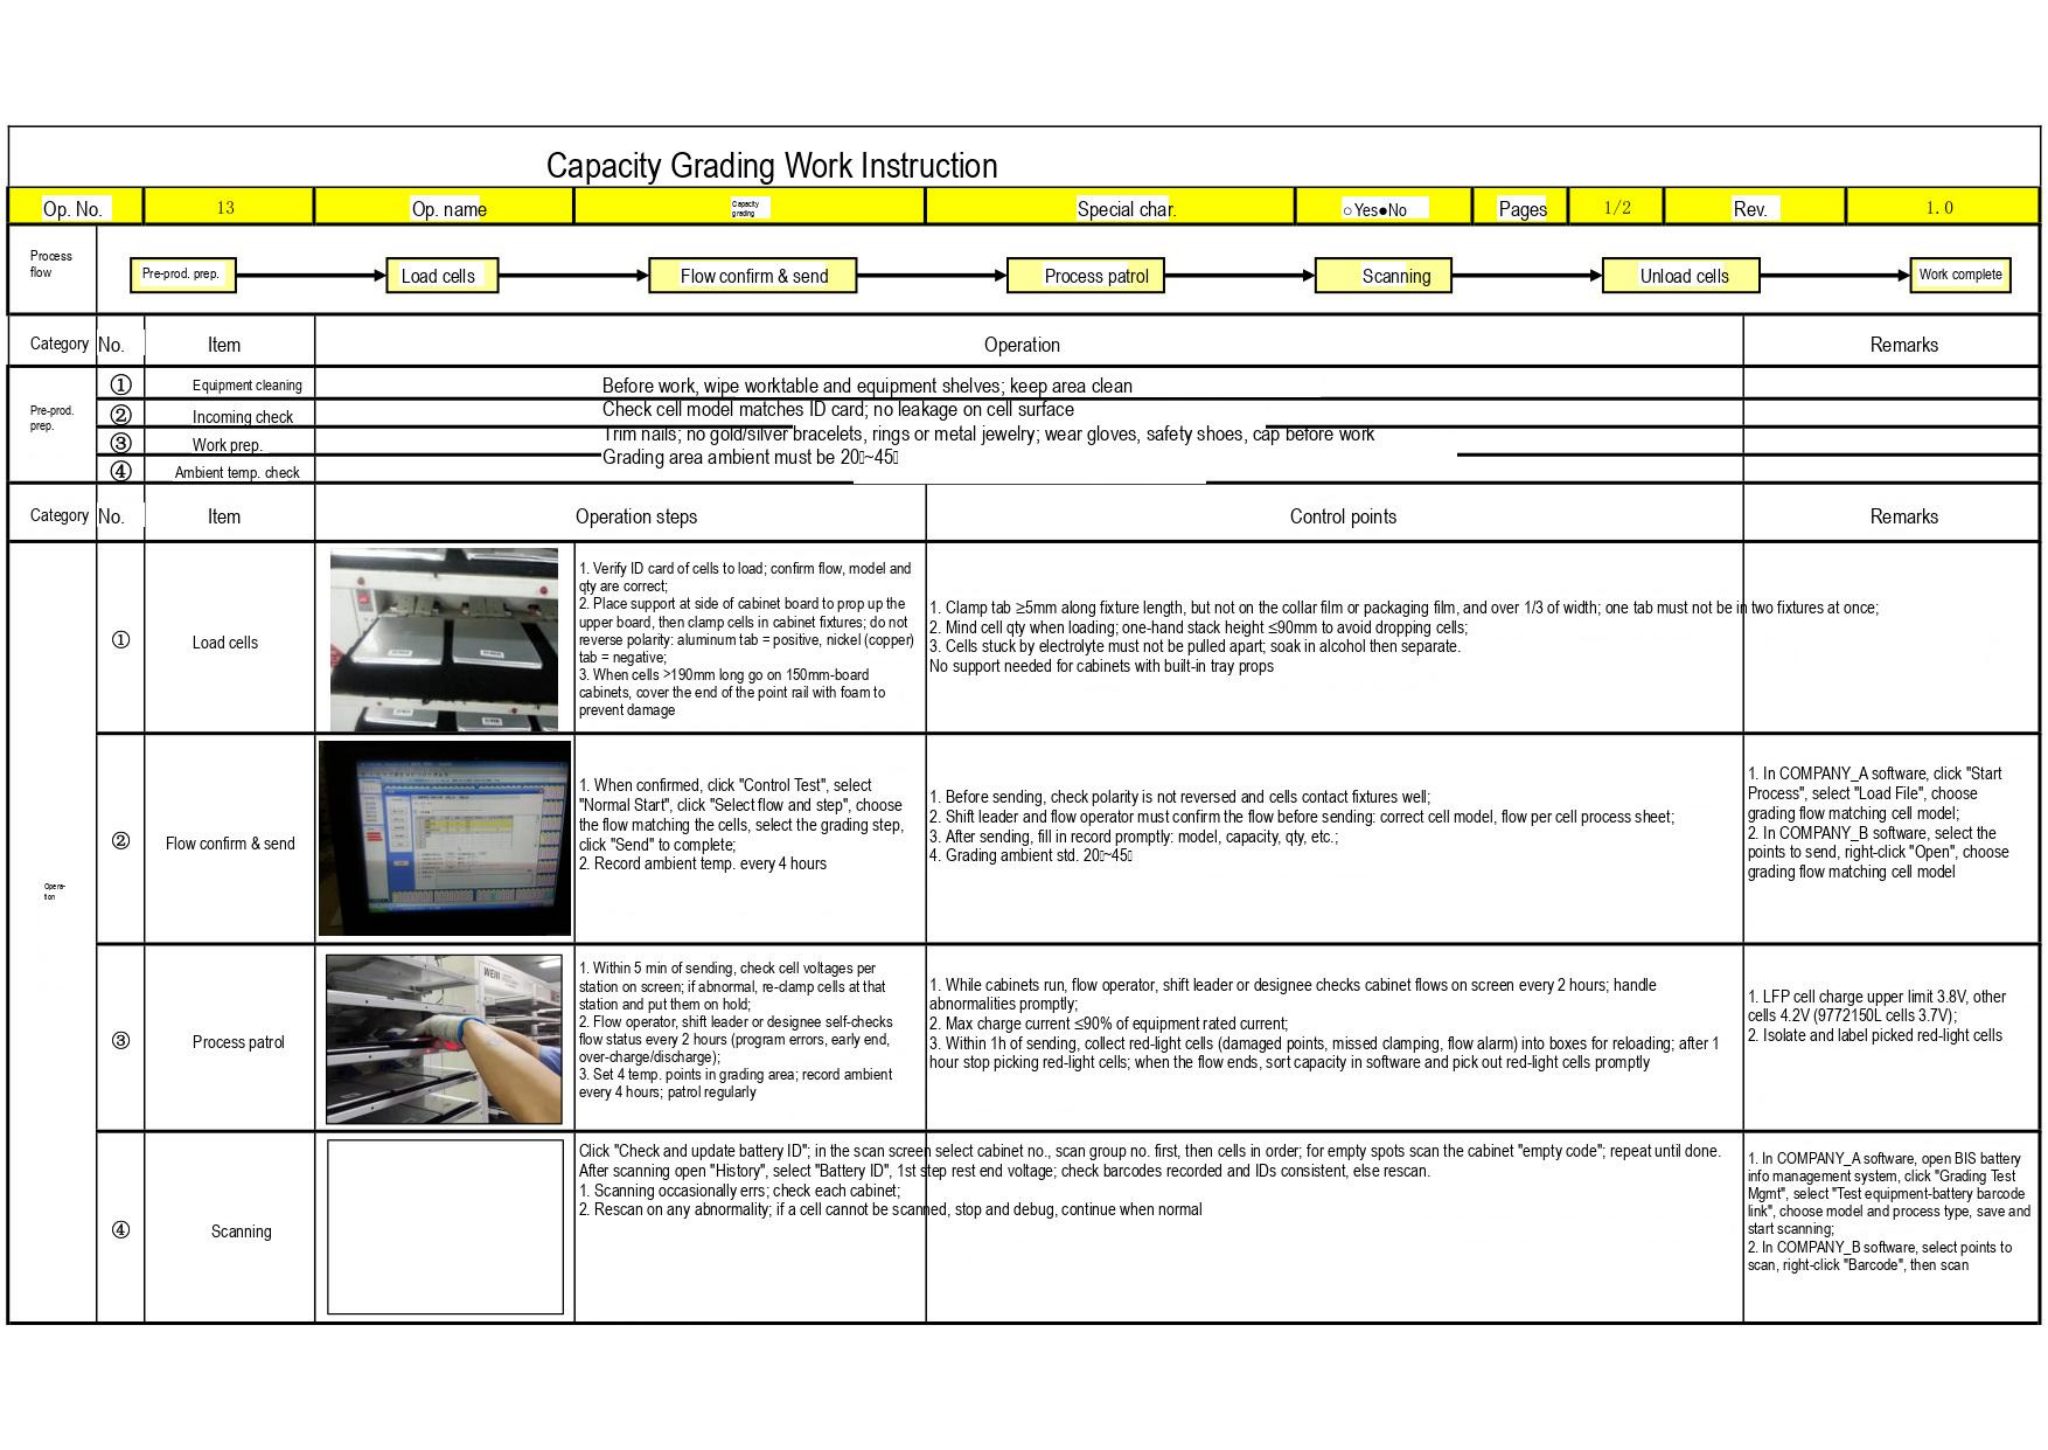# Capacity Grading Work Instruction

| Op. No. | 13 | Op. name | Capacity grading | Special char. | ○Yes●No | Pages | 1/2 | Rev. | 1.0 |
|---|---|---|---|---|---|---|---|---|---|

Process flow: Pre-prod. prep. → Load cells → Flow confirm & send → Process patrol → Scanning → Unload cells → Work complete

| Category | No. | Item | Operation | Remarks |
|---|---|---|---|---|
| Pre-prod. prep. | ① | Equipment cleaning | Before work, wipe worktable and equipment shelves; keep area clean | |
| | ② | Incoming check | Check cell model matches ID card; no leakage on cell surface | |
| | ③ | Work prep. | Trim nails; no gold/silver bracelets, rings or metal jewelry; wear gloves, safety shoes, cap before work | |
| | ④ | Ambient temp. check | Grading area ambient must be 20~45 | |

| Category | No. | Item | Operation steps | | Control points | Remarks |
|---|---|---|---|---|---|---|
| Operation | ① | Load cells | | 1. Verify ID card of cells to load; confirm flow, model and qty are correct;<br>2. Place support at side of cabinet board to prop up the upper board, then clamp cells in cabinet fixtures; do not reverse polarity: aluminum tab = positive, nickel (copper) tab = negative;<br>3. When cells >190mm long go on 150mm-board cabinets, cover the end of the point rail with foam to prevent damage | 1. Clamp tab ≥5mm along fixture length, but not on the collar film or packaging film, and over 1/3 of width; one tab must not be in two fixtures at once;<br>2. Mind cell qty when loading; one-hand stack height ≤90mm to avoid dropping cells;<br>3. Cells stuck by electrolyte must not be pulled apart; soak in alcohol then separate.<br>No support needed for cabinets with built-in tray props | |
| | ② | Flow confirm & send | | 1. When confirmed, click "Control Test", select "Normal Start", click "Select flow and step", choose the flow matching the cells, select the grading step, click "Send" to complete;<br>2. Record ambient temp. every 4 hours | 1. Before sending, check polarity is not reversed and cells contact fixtures well;<br>2. Shift leader and flow operator must confirm the flow before sending: correct cell model, flow per cell process sheet;<br>3. After sending, fill in record promptly: model, capacity, qty, etc.;<br>4. Grading ambient std. 20~45 | 1. In COMPANY_A software, click "Start Process", select "Load File", choose grading flow matching cell model;<br>2. In COMPANY_B software, select the points to send, right-click "Open", choose grading flow matching cell model |
| | ③ | Process patrol | | 1. Within 5 min of sending, check cell voltages per station on screen; if abnormal, re-clamp cells at that station and put them on hold;<br>2. Flow operator, shift leader or designee self-checks flow status every 2 hours (program errors, early end, over-charge/discharge);<br>3. Set 4 temp. points in grading area; record ambient every 4 hours; patrol regularly | 1. While cabinets run, flow operator, shift leader or designee checks cabinet flows on screen every 2 hours; handle abnormalities promptly;<br>2. Max charge current ≤90% of equipment rated current;<br>3. Within 1h of sending, collect red-light cells (damaged points, missed clamping, flow alarm) into boxes for reloading; after 1 hour stop picking red-light cells; when the flow ends, sort capacity in software and pick out red-light cells promptly | 1. LFP cell charge upper limit 3.8V, other cells 4.2V (9772150L cells 3.7V);<br>2. Isolate and label picked red-light cells |
| | ④ | Scanning | | Click "Check and update battery ID"; in the scan screen select cabinet no., scan group no. first, then cells in order; for empty spots scan the cabinet "empty code"; repeat until done. After scanning open "History", select "Battery ID", 1st step rest end voltage; check barcodes recorded and IDs consistent, else rescan.<br>1. Scanning occasionally errs; check each cabinet;<br>2. Rescan on any abnormality; if a cell cannot be scanned, stop and debug, continue when normal | | 1. In COMPANY_A software, open BIS battery info management system, click "Grading Test Mgmt", select "Test equipment-battery barcode link", choose model and process type, save and start scanning;<br>2. In COMPANY_B software, select points to scan, right-click "Barcode", then scan |

WEIR
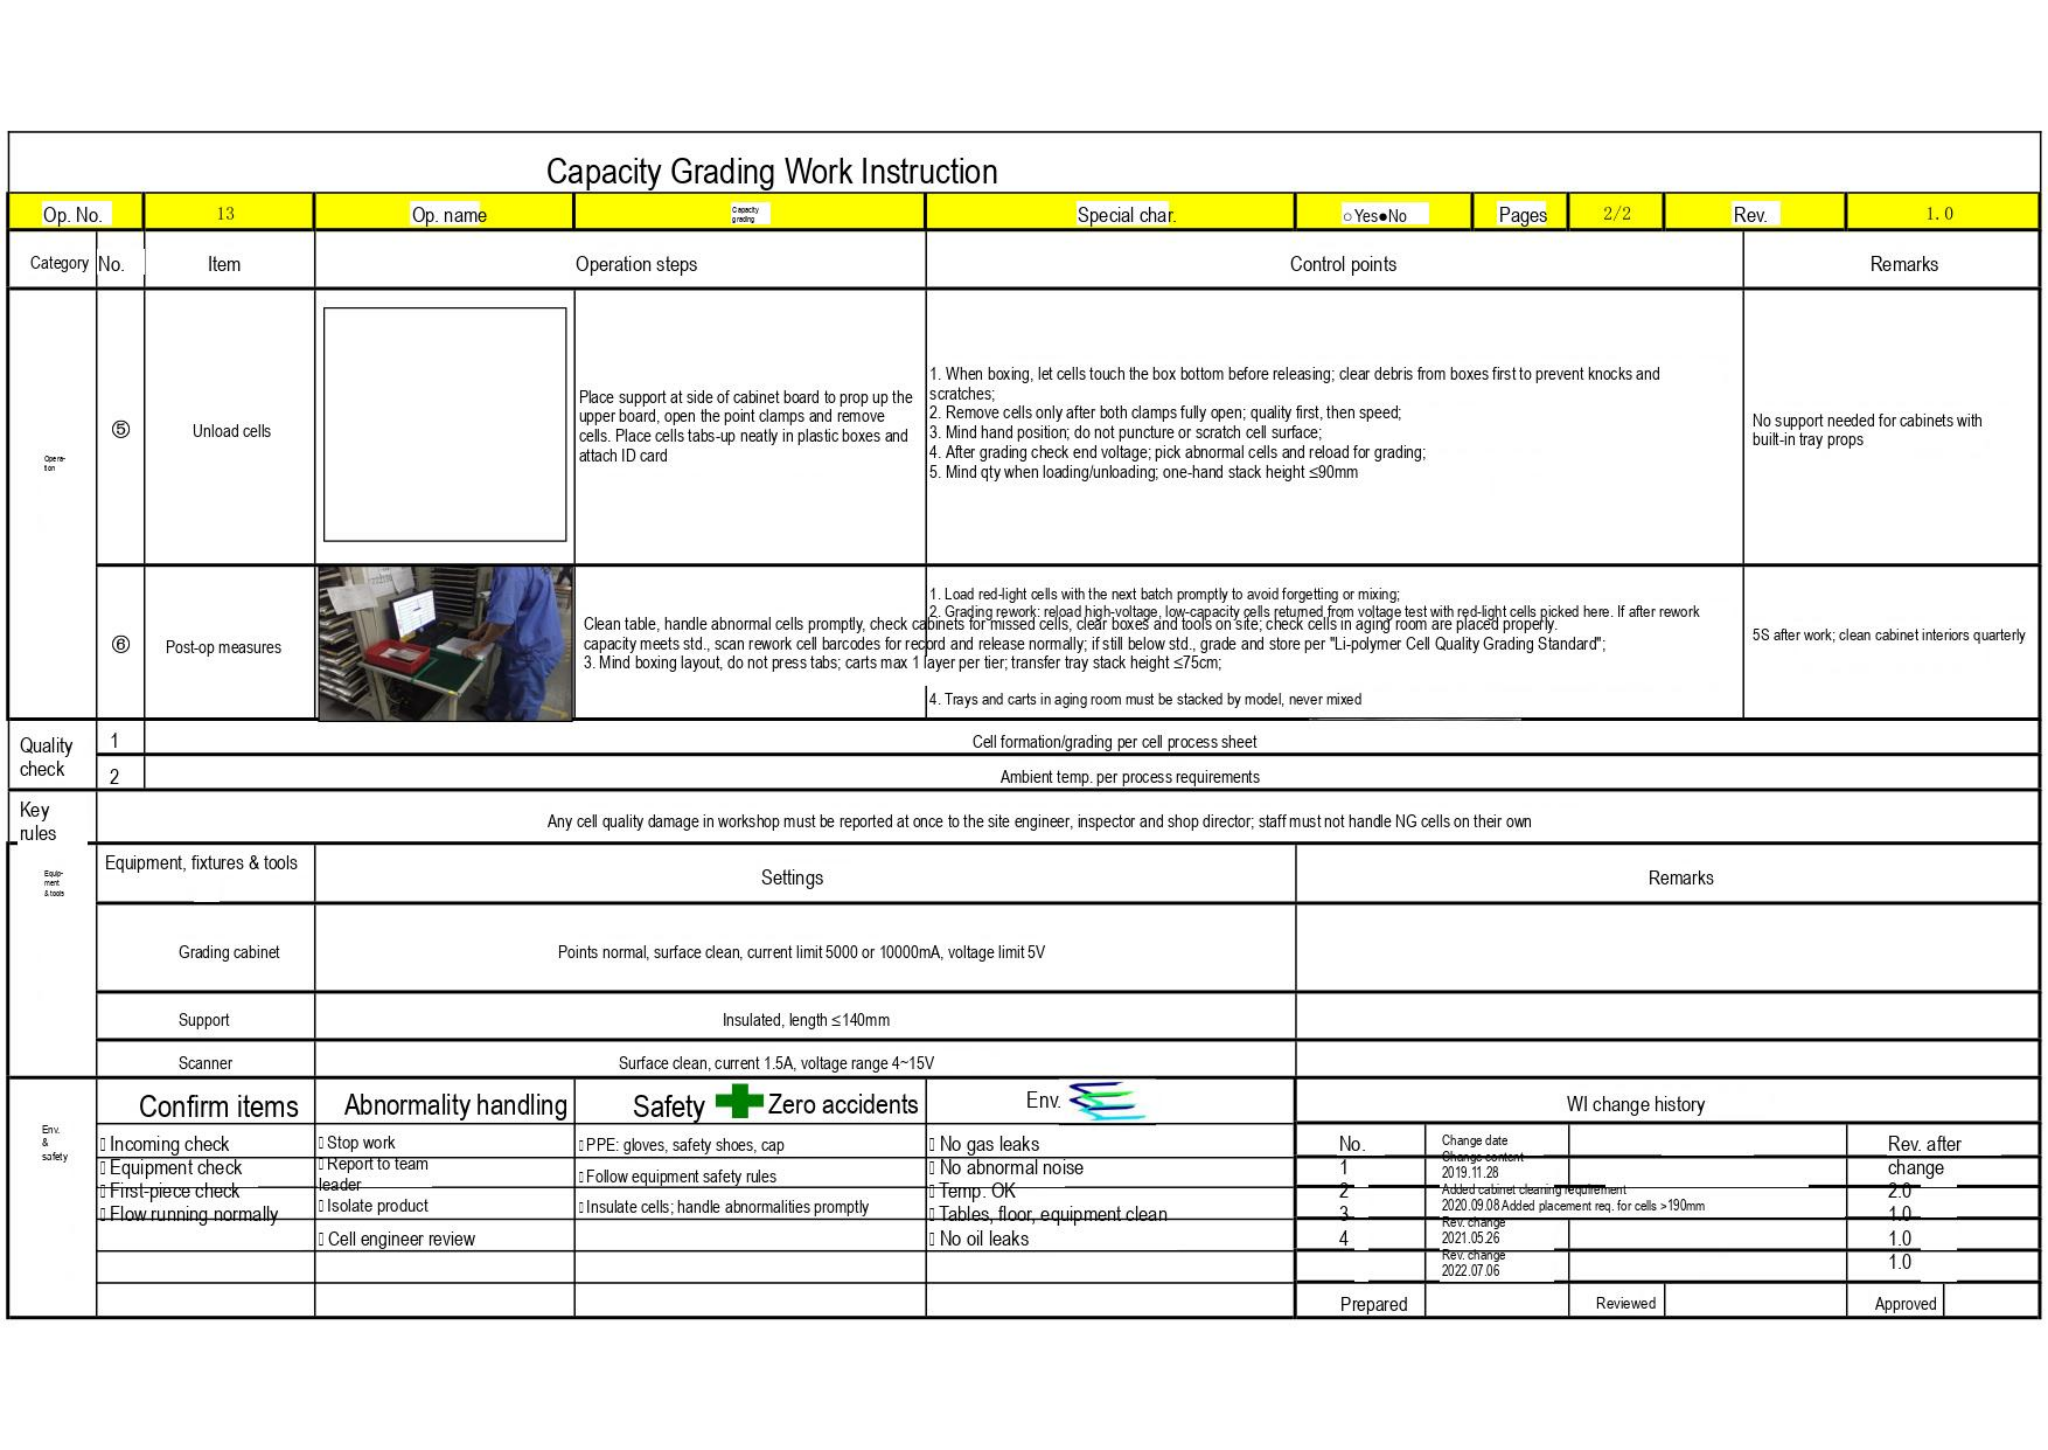# Capacity Grading Work Instruction

| Op. No. | 13 | Op. name | Capacity grading | Special char. | ○Yes●No | Pages | 2/2 | Rev. | 1.0 |
|---|---|---|---|---|---|---|---|---|---|

| Category | No. | Item | Operation steps | Control points | Remarks |
|---|---|---|---|---|---|
| Opera-tion | ⑤ | Unload cells | Place support at side of cabinet board to prop up the upper board, open the point clamps and remove cells. Place cells tabs-up neatly in plastic boxes and attach ID card | 1. When boxing, let cells touch the box bottom before releasing; clear debris from boxes first to prevent knocks and scratches;<br>2. Remove cells only after both clamps fully open; quality first, then speed;<br>3. Mind hand position; do not puncture or scratch cell surface;<br>4. After grading check end voltage; pick abnormal cells and reload for grading;<br>5. Mind qty when loading/unloading; one-hand stack height ≤90mm | No support needed for cabinets with built-in tray props |
| | ⑥ | Post-op measures | Clean table, handle abnormal cells promptly, check cabinets for missed cells, clear boxes and tools on site; check cells in aging room are placed properly. | 1. Load red-light cells with the next batch promptly to avoid forgetting or mixing;<br>2. Grading rework: reload high-voltage, low-capacity cells returned from voltage test with red-light cells picked here. If after rework capacity meets std., scan rework cell barcodes for record and release normally; if still below std., grade and store per "Li-polymer Cell Quality Grading Standard";<br>3. Mind boxing layout, do not press tabs; carts max 1 layer per tier; transfer tray stack height ≤75cm;<br>4. Trays and carts in aging room must be stacked by model, never mixed | 5S after work; clean cabinet interiors quarterly |

| Quality check | | |
|---|---|---|
| | 1 | Cell formation/grading per cell process sheet |
| | 2 | Ambient temp. per process requirements |

| Key rules | Any cell quality damage in workshop must be reported at once to the site engineer, inspector and shop director; staff must not handle NG cells on their own |
|---|---|

| Equip-ment & tools | Equipment, fixtures & tools | Settings | Remarks |
|---|---|---|---|
| | Grading cabinet | Points normal, surface clean, current limit 5000 or 10000mA, voltage limit 5V | |
| | Support | Insulated, length ≤140mm | |
| | Scanner | Surface clean, current 1.5A, voltage range 4~15V | |

| Env. & safety | Confirm items | Abnormality handling | Safety Zero accidents | Env. |
|---|---|---|---|---|
| | □ Incoming check | □ Stop work | □ PPE: gloves, safety shoes, cap | □ No gas leaks |
| | □ Equipment check | □ Report to team leader | □ Follow equipment safety rules | □ No abnormal noise |
| | □ First-piece check | □ Isolate product | □ Insulate cells; handle abnormalities promptly | □ Temp. OK |
| | □ Flow running normally | | | □ Tables, floor, equipment clean |
| | | □ Cell engineer review | | □ No oil leaks |

WI change history

| No. | Change date / Change content | | Rev. after change |
|---|---|---|---|
| 1 | 2019.11.28 | | |
| 2 | Added cabinet cleaning requirement | | 2.0 |
| 3 | 2020.09.08 Added placement req. for cells >190mm | | 1.0 |
| 4 | Rev. change 2021.05.26 | | 1.0 |
| | Rev. change 2022.07.06 | | 1.0 |
| Prepared | | Reviewed | Approved |